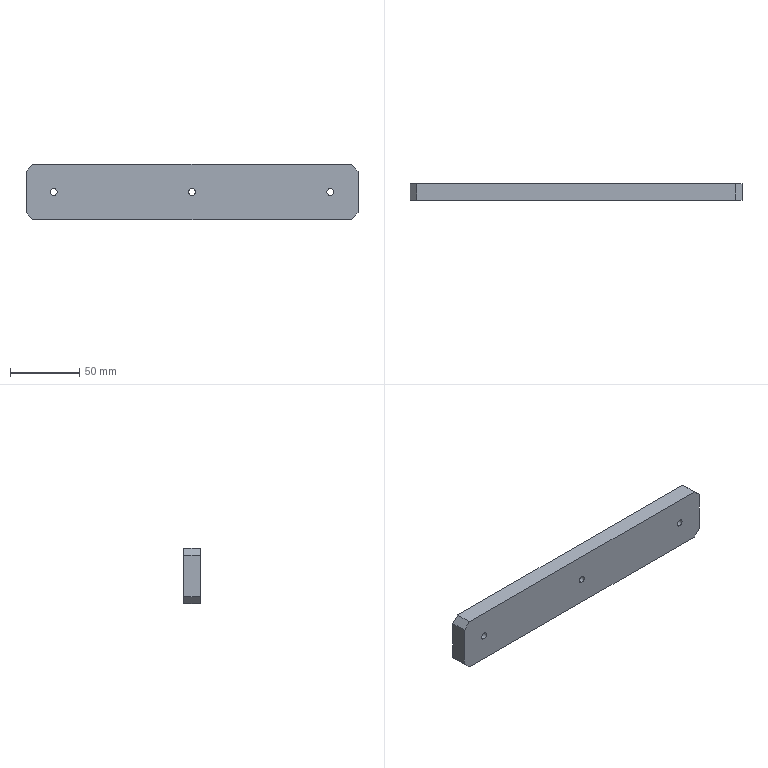Part | SolidWorks | features Chamfer 1, Extrusion 1, HoleWzd 1 | 1 solid | 16 faces | box 240 x 12 x 40 mm | volume 113893 mm3 | plane 10 | cylinder 6 | commonest cylinder face diameters 5 x6
STEP:
#1=CARTESIAN_POINT('',(-100.,-6.,-2.5));
#2=VERTEX_POINT('',#1);
#3=CARTESIAN_POINT('',(-100.,-6.,2.5));
#4=VERTEX_POINT('',#3);
#5=CARTESIAN_POINT('',(-100.,-6.,0.));
#6=DIRECTION('',(0.,1.,0.));
#7=DIRECTION('',(0.,0.,1.));
#8=AXIS2_PLACEMENT_3D('',#5,#6,#7);
#9=CIRCLE('',#8,2.5);
#10=EDGE_CURVE('',#2,#4,#9,.T.);
#11=ORIENTED_EDGE('',*,*,#10,.F.);
#12=CARTESIAN_POINT('',(-100.,6.,-2.5));
#13=VERTEX_POINT('',#12);
#14=CARTESIAN_POINT('',(-100.,6.,-2.5));
#15=DIRECTION('',(0.,1.,0.));
#16=VECTOR('',#15,1000.);
#17=LINE('',#14,#16);
#18=EDGE_CURVE('',#2,#13,#17,.T.);
#19=ORIENTED_EDGE('',*,*,#18,.T.);
#20=CARTESIAN_POINT('',(-100.,6.,2.5));
#21=VERTEX_POINT('',#20);
#22=CARTESIAN_POINT('',(-100.,6.,0.));
#23=DIRECTION('',(0.,1.,0.));
#24=DIRECTION('',(0.,0.,1.));
#25=AXIS2_PLACEMENT_3D('',#22,#23,#24);
#26=CIRCLE('',#25,2.5);
#27=EDGE_CURVE('',#13,#21,#26,.T.);
#28=ORIENTED_EDGE('',*,*,#27,.T.);
#29=CARTESIAN_POINT('',(-100.,6.,2.5));
#30=DIRECTION('',(0.,1.,0.));
#31=VECTOR('',#30,1000.);
#32=LINE('',#29,#31);
#33=EDGE_CURVE('',#4,#21,#32,.T.);
#34=ORIENTED_EDGE('',*,*,#33,.F.);
#35=EDGE_LOOP('',(#11,#19,#28,#34));
#36=FACE_OUTER_BOUND('',#35,.T.);
#37=CARTESIAN_POINT('',(-100.,6.,0.));
#38=DIRECTION('',(0.,1.,0.));
#39=DIRECTION('',(0.,0.,1.));
#40=AXIS2_PLACEMENT_3D('',#37,#38,#39);
#41=CYLINDRICAL_SURFACE('',#40,2.5);
#42=ADVANCED_FACE('',(#36),#41,.F.);
#43=CARTESIAN_POINT('',(0.,-6.,-2.5));
#44=VERTEX_POINT('',#43);
#45=CARTESIAN_POINT('',(0.,-6.,2.5));
#46=VERTEX_POINT('',#45);
#47=CARTESIAN_POINT('',(0.,-6.,0.));
#48=DIRECTION('',(0.,1.,0.));
#49=DIRECTION('',(0.,0.,1.));
#50=AXIS2_PLACEMENT_3D('',#47,#48,#49);
#51=CIRCLE('',#50,2.5);
#52=EDGE_CURVE('',#44,#46,#51,.T.);
#53=ORIENTED_EDGE('',*,*,#52,.F.);
#54=CARTESIAN_POINT('',(0.,6.,-2.5));
#55=VERTEX_POINT('',#54);
#56=CARTESIAN_POINT('',(0.,6.,-2.5));
#57=DIRECTION('',(0.,1.,0.));
#58=VECTOR('',#57,1000.);
#59=LINE('',#56,#58);
#60=EDGE_CURVE('',#44,#55,#59,.T.);
#61=ORIENTED_EDGE('',*,*,#60,.T.);
#62=CARTESIAN_POINT('',(0.,6.,2.5));
#63=VERTEX_POINT('',#62);
#64=CARTESIAN_POINT('',(0.,6.,0.));
#65=DIRECTION('',(0.,1.,0.));
#66=DIRECTION('',(0.,0.,1.));
#67=AXIS2_PLACEMENT_3D('',#64,#65,#66);
#68=CIRCLE('',#67,2.5);
#69=EDGE_CURVE('',#55,#63,#68,.T.);
#70=ORIENTED_EDGE('',*,*,#69,.T.);
#71=CARTESIAN_POINT('',(0.,6.,2.5));
#72=DIRECTION('',(0.,1.,0.));
#73=VECTOR('',#72,1000.);
#74=LINE('',#71,#73);
#75=EDGE_CURVE('',#46,#63,#74,.T.);
#76=ORIENTED_EDGE('',*,*,#75,.F.);
#77=EDGE_LOOP('',(#53,#61,#70,#76));
#78=FACE_OUTER_BOUND('',#77,.T.);
#79=CARTESIAN_POINT('',(0.,6.,0.));
#80=DIRECTION('',(0.,1.,0.));
#81=DIRECTION('',(0.,0.,1.));
#82=AXIS2_PLACEMENT_3D('',#79,#80,#81);
#83=CYLINDRICAL_SURFACE('',#82,2.5);
#84=ADVANCED_FACE('',(#78),#83,.F.);
#85=CARTESIAN_POINT('',(100.,-6.,-2.5));
#86=VERTEX_POINT('',#85);
#87=CARTESIAN_POINT('',(100.,-6.,2.5));
#88=VERTEX_POINT('',#87);
#89=CARTESIAN_POINT('',(100.,-6.,0.));
#90=DIRECTION('',(0.,1.,0.));
#91=DIRECTION('',(0.,0.,1.));
#92=AXIS2_PLACEMENT_3D('',#89,#90,#91);
#93=CIRCLE('',#92,2.5);
#94=EDGE_CURVE('',#86,#88,#93,.T.);
#95=ORIENTED_EDGE('',*,*,#94,.F.);
#96=CARTESIAN_POINT('',(100.,6.,-2.5));
#97=VERTEX_POINT('',#96);
#98=CARTESIAN_POINT('',(100.,6.,-2.5));
#99=DIRECTION('',(0.,1.,0.));
#100=VECTOR('',#99,1000.);
#101=LINE('',#98,#100);
#102=EDGE_CURVE('',#86,#97,#101,.T.);
#103=ORIENTED_EDGE('',*,*,#102,.T.);
#104=CARTESIAN_POINT('',(100.,6.,2.5));
#105=VERTEX_POINT('',#104);
#106=CARTESIAN_POINT('',(100.,6.,0.));
#107=DIRECTION('',(0.,1.,0.));
#108=DIRECTION('',(0.,0.,1.));
#109=AXIS2_PLACEMENT_3D('',#106,#107,#108);
#110=CIRCLE('',#109,2.5);
#111=EDGE_CURVE('',#97,#105,#110,.T.);
#112=ORIENTED_EDGE('',*,*,#111,.T.);
#113=CARTESIAN_POINT('',(100.,6.,2.5));
#114=DIRECTION('',(0.,1.,0.));
#115=VECTOR('',#114,1000.);
#116=LINE('',#113,#115);
#117=EDGE_CURVE('',#88,#105,#116,.T.);
#118=ORIENTED_EDGE('',*,*,#117,.F.);
#119=EDGE_LOOP('',(#95,#103,#112,#118));
#120=FACE_OUTER_BOUND('',#119,.T.);
#121=CARTESIAN_POINT('',(100.,6.,0.));
#122=DIRECTION('',(0.,1.,0.));
#123=DIRECTION('',(0.,0.,1.));
#124=AXIS2_PLACEMENT_3D('',#121,#122,#123);
#125=CYLINDRICAL_SURFACE('',#124,2.5);
#126=ADVANCED_FACE('',(#120),#125,.F.);
#127=CARTESIAN_POINT('',(-120.,-6.,-15.));
#128=VERTEX_POINT('',#127);
#129=CARTESIAN_POINT('',(-120.,-6.,15.));
#130=VERTEX_POINT('',#129);
#131=CARTESIAN_POINT('',(-120.,-6.,-20.));
#132=DIRECTION('',(0.,0.,1.));
#133=VECTOR('',#132,1000.);
#134=LINE('',#131,#133);
#135=EDGE_CURVE('',#128,#130,#134,.T.);
#136=ORIENTED_EDGE('',*,*,#135,.T.);
#137=CARTESIAN_POINT('',(-120.,6.,15.));
#138=VERTEX_POINT('',#137);
#139=CARTESIAN_POINT('',(-120.,6.,15.));
#140=DIRECTION('',(0.,1.,0.));
#141=VECTOR('',#140,1000.);
#142=LINE('',#139,#141);
#143=EDGE_CURVE('',#130,#138,#142,.T.);
#144=ORIENTED_EDGE('',*,*,#143,.T.);
#145=CARTESIAN_POINT('',(-120.,6.,-15.));
#146=VERTEX_POINT('',#145);
#147=CARTESIAN_POINT('',(-120.,6.,-20.));
#148=DIRECTION('',(0.,0.,1.));
#149=VECTOR('',#148,1000.);
#150=LINE('',#147,#149);
#151=EDGE_CURVE('',#146,#138,#150,.T.);
#152=ORIENTED_EDGE('',*,*,#151,.F.);
#153=CARTESIAN_POINT('',(-120.,6.,-15.));
#154=DIRECTION('',(0.,-1.,0.));
#155=VECTOR('',#154,1000.);
#156=LINE('',#153,#155);
#157=EDGE_CURVE('',#146,#128,#156,.T.);
#158=ORIENTED_EDGE('',*,*,#157,.T.);
#159=EDGE_LOOP('',(#136,#144,#152,#158));
#160=FACE_OUTER_BOUND('',#159,.T.);
#161=CARTESIAN_POINT('',(-120.,6.,-20.));
#162=DIRECTION('',(1.,0.,0.));
#163=DIRECTION('',(0.,0.,-1.));
#164=AXIS2_PLACEMENT_3D('',#161,#162,#163);
#165=PLANE('',#164);
#166=ADVANCED_FACE('',(#160),#165,.F.);
#167=CARTESIAN_POINT('',(-115.,-6.,20.));
#168=VERTEX_POINT('',#167);
#169=CARTESIAN_POINT('',(115.,-6.,20.));
#170=VERTEX_POINT('',#169);
#171=CARTESIAN_POINT('',(-120.,-6.,20.));
#172=DIRECTION('',(1.,0.,0.));
#173=VECTOR('',#172,1000.);
#174=LINE('',#171,#173);
#175=EDGE_CURVE('',#168,#170,#174,.T.);
#176=ORIENTED_EDGE('',*,*,#175,.T.);
#177=CARTESIAN_POINT('',(115.,6.,20.));
#178=VERTEX_POINT('',#177);
#179=CARTESIAN_POINT('',(115.,6.,20.));
#180=DIRECTION('',(0.,1.,0.));
#181=VECTOR('',#180,1000.);
#182=LINE('',#179,#181);
#183=EDGE_CURVE('',#170,#178,#182,.T.);
#184=ORIENTED_EDGE('',*,*,#183,.T.);
#185=CARTESIAN_POINT('',(-115.,6.,20.));
#186=VERTEX_POINT('',#185);
#187=CARTESIAN_POINT('',(-120.,6.,20.));
#188=DIRECTION('',(1.,0.,0.));
#189=VECTOR('',#188,1000.);
#190=LINE('',#187,#189);
#191=EDGE_CURVE('',#186,#178,#190,.T.);
#192=ORIENTED_EDGE('',*,*,#191,.F.);
#193=CARTESIAN_POINT('',(-115.,6.,20.));
#194=DIRECTION('',(0.,-1.,0.));
#195=VECTOR('',#194,1000.);
#196=LINE('',#193,#195);
#197=EDGE_CURVE('',#186,#168,#196,.T.);
#198=ORIENTED_EDGE('',*,*,#197,.T.);
#199=EDGE_LOOP('',(#176,#184,#192,#198));
#200=FACE_OUTER_BOUND('',#199,.T.);
#201=CARTESIAN_POINT('',(-120.,6.,20.));
#202=DIRECTION('',(0.,0.,-1.));
#203=DIRECTION('',(-1.,0.,0.));
#204=AXIS2_PLACEMENT_3D('',#201,#202,#203);
#205=PLANE('',#204);
#206=ADVANCED_FACE('',(#200),#205,.F.);
#207=CARTESIAN_POINT('',(120.,6.,15.));
#208=VERTEX_POINT('',#207);
#209=CARTESIAN_POINT('',(120.,6.,-15.));
#210=VERTEX_POINT('',#209);
#211=CARTESIAN_POINT('',(120.,6.,-20.));
#212=DIRECTION('',(0.,0.,-1.));
#213=VECTOR('',#212,1000.);
#214=LINE('',#211,#213);
#215=EDGE_CURVE('',#208,#210,#214,.T.);
#216=ORIENTED_EDGE('',*,*,#215,.F.);
#217=CARTESIAN_POINT('',(120.,-6.,15.));
#218=VERTEX_POINT('',#217);
#219=CARTESIAN_POINT('',(120.,6.,15.));
#220=DIRECTION('',(0.,-1.,0.));
#221=VECTOR('',#220,1000.);
#222=LINE('',#219,#221);
#223=EDGE_CURVE('',#208,#218,#222,.T.);
#224=ORIENTED_EDGE('',*,*,#223,.T.);
#225=CARTESIAN_POINT('',(120.,-6.,-15.));
#226=VERTEX_POINT('',#225);
#227=CARTESIAN_POINT('',(120.,-6.,-20.));
#228=DIRECTION('',(0.,0.,-1.));
#229=VECTOR('',#228,1000.);
#230=LINE('',#227,#229);
#231=EDGE_CURVE('',#218,#226,#230,.T.);
#232=ORIENTED_EDGE('',*,*,#231,.T.);
#233=CARTESIAN_POINT('',(120.,6.,-15.));
#234=DIRECTION('',(0.,1.,0.));
#235=VECTOR('',#234,1000.);
#236=LINE('',#233,#235);
#237=EDGE_CURVE('',#226,#210,#236,.T.);
#238=ORIENTED_EDGE('',*,*,#237,.T.);
#239=EDGE_LOOP('',(#216,#224,#232,#238));
#240=FACE_OUTER_BOUND('',#239,.T.);
#241=CARTESIAN_POINT('',(120.,6.,-20.));
#242=DIRECTION('',(-1.,0.,0.));
#243=DIRECTION('',(0.,0.,1.));
#244=AXIS2_PLACEMENT_3D('',#241,#242,#243);
#245=PLANE('',#244);
#246=ADVANCED_FACE('',(#240),#245,.F.);
#247=CARTESIAN_POINT('',(115.,-6.,-20.));
#248=VERTEX_POINT('',#247);
#249=CARTESIAN_POINT('',(-115.,-6.,-20.));
#250=VERTEX_POINT('',#249);
#251=CARTESIAN_POINT('',(-120.,-6.,-20.));
#252=DIRECTION('',(-1.,0.,0.));
#253=VECTOR('',#252,1000.);
#254=LINE('',#251,#253);
#255=EDGE_CURVE('',#248,#250,#254,.T.);
#256=ORIENTED_EDGE('',*,*,#255,.T.);
#257=CARTESIAN_POINT('',(-115.,6.,-20.));
#258=VERTEX_POINT('',#257);
#259=CARTESIAN_POINT('',(-115.,6.,-20.));
#260=DIRECTION('',(0.,1.,0.));
#261=VECTOR('',#260,1000.);
#262=LINE('',#259,#261);
#263=EDGE_CURVE('',#250,#258,#262,.T.);
#264=ORIENTED_EDGE('',*,*,#263,.T.);
#265=CARTESIAN_POINT('',(115.,6.,-20.));
#266=VERTEX_POINT('',#265);
#267=CARTESIAN_POINT('',(-120.,6.,-20.));
#268=DIRECTION('',(-1.,0.,0.));
#269=VECTOR('',#268,1000.);
#270=LINE('',#267,#269);
#271=EDGE_CURVE('',#266,#258,#270,.T.);
#272=ORIENTED_EDGE('',*,*,#271,.F.);
#273=CARTESIAN_POINT('',(115.,6.,-20.));
#274=DIRECTION('',(0.,-1.,0.));
#275=VECTOR('',#274,1000.);
#276=LINE('',#273,#275);
#277=EDGE_CURVE('',#266,#248,#276,.T.);
#278=ORIENTED_EDGE('',*,*,#277,.T.);
#279=EDGE_LOOP('',(#256,#264,#272,#278));
#280=FACE_OUTER_BOUND('',#279,.T.);
#281=CARTESIAN_POINT('',(-120.,6.,-20.));
#282=DIRECTION('',(0.,0.,1.));
#283=DIRECTION('',(1.,0.,0.));
#284=AXIS2_PLACEMENT_3D('',#281,#282,#283);
#285=PLANE('',#284);
#286=ADVANCED_FACE('',(#280),#285,.F.);
#287=CARTESIAN_POINT('',(-100.,6.,0.));
#288=DIRECTION('',(0.,1.,0.));
#289=DIRECTION('',(0.,0.,1.));
#290=AXIS2_PLACEMENT_3D('',#287,#288,#289);
#291=CIRCLE('',#290,2.5);
#292=EDGE_CURVE('',#21,#13,#291,.T.);
#293=ORIENTED_EDGE('',*,*,#292,.F.);
#294=ORIENTED_EDGE('',*,*,#27,.F.);
#295=EDGE_LOOP('',(#293,#294));
#296=FACE_BOUND('',#295,.T.);
#297=CARTESIAN_POINT('',(0.,6.,0.));
#298=DIRECTION('',(0.,1.,0.));
#299=DIRECTION('',(0.,0.,1.));
#300=AXIS2_PLACEMENT_3D('',#297,#298,#299);
#301=CIRCLE('',#300,2.5);
#302=EDGE_CURVE('',#63,#55,#301,.T.);
#303=ORIENTED_EDGE('',*,*,#302,.F.);
#304=ORIENTED_EDGE('',*,*,#69,.F.);
#305=EDGE_LOOP('',(#303,#304));
#306=FACE_BOUND('',#305,.T.);
#307=CARTESIAN_POINT('',(100.,6.,0.));
#308=DIRECTION('',(0.,1.,0.));
#309=DIRECTION('',(0.,0.,1.));
#310=AXIS2_PLACEMENT_3D('',#307,#308,#309);
#311=CIRCLE('',#310,2.5);
#312=EDGE_CURVE('',#105,#97,#311,.T.);
#313=ORIENTED_EDGE('',*,*,#312,.F.);
#314=ORIENTED_EDGE('',*,*,#111,.F.);
#315=EDGE_LOOP('',(#313,#314));
#316=FACE_BOUND('',#315,.T.);
#317=ORIENTED_EDGE('',*,*,#191,.T.);
#318=CARTESIAN_POINT('',(-2.5,6.,137.5));
#319=DIRECTION('',(0.7071,0.,-0.7071));
#320=VECTOR('',#319,1000.);
#321=LINE('',#318,#320);
#322=EDGE_CURVE('',#178,#208,#321,.T.);
#323=ORIENTED_EDGE('',*,*,#322,.T.);
#324=ORIENTED_EDGE('',*,*,#215,.T.);
#325=CARTESIAN_POINT('',(17.5,6.,-117.5));
#326=DIRECTION('',(-0.7071,0.,-0.7071));
#327=VECTOR('',#326,1000.);
#328=LINE('',#325,#327);
#329=EDGE_CURVE('',#210,#266,#328,.T.);
#330=ORIENTED_EDGE('',*,*,#329,.T.);
#331=ORIENTED_EDGE('',*,*,#271,.T.);
#332=CARTESIAN_POINT('',(-137.5,6.,2.5));
#333=DIRECTION('',(-0.7071,0.,0.7071));
#334=VECTOR('',#333,1000.);
#335=LINE('',#332,#334);
#336=EDGE_CURVE('',#258,#146,#335,.T.);
#337=ORIENTED_EDGE('',*,*,#336,.T.);
#338=ORIENTED_EDGE('',*,*,#151,.T.);
#339=CARTESIAN_POINT('',(-117.5,6.,17.5));
#340=DIRECTION('',(0.7071,0.,0.7071));
#341=VECTOR('',#340,1000.);
#342=LINE('',#339,#341);
#343=EDGE_CURVE('',#138,#186,#342,.T.);
#344=ORIENTED_EDGE('',*,*,#343,.T.);
#345=EDGE_LOOP('',(#317,#323,#324,#330,#331,#337,#338,#344));
#346=FACE_OUTER_BOUND('',#345,.T.);
#347=CARTESIAN_POINT('',(-120.,6.,20.));
#348=DIRECTION('',(0.,1.,0.));
#349=DIRECTION('',(0.,0.,1.));
#350=AXIS2_PLACEMENT_3D('',#347,#348,#349);
#351=PLANE('',#350);
#352=ADVANCED_FACE('',(#296,#306,#316,#346),#351,.T.);
#353=CARTESIAN_POINT('',(-100.,-6.,0.));
#354=DIRECTION('',(0.,1.,0.));
#355=DIRECTION('',(0.,0.,1.));
#356=AXIS2_PLACEMENT_3D('',#353,#354,#355);
#357=CIRCLE('',#356,2.5);
#358=EDGE_CURVE('',#4,#2,#357,.T.);
#359=ORIENTED_EDGE('',*,*,#358,.T.);
#360=ORIENTED_EDGE('',*,*,#10,.T.);
#361=EDGE_LOOP('',(#359,#360));
#362=FACE_BOUND('',#361,.T.);
#363=CARTESIAN_POINT('',(0.,-6.,0.));
#364=DIRECTION('',(0.,1.,0.));
#365=DIRECTION('',(0.,0.,1.));
#366=AXIS2_PLACEMENT_3D('',#363,#364,#365);
#367=CIRCLE('',#366,2.5);
#368=EDGE_CURVE('',#46,#44,#367,.T.);
#369=ORIENTED_EDGE('',*,*,#368,.T.);
#370=ORIENTED_EDGE('',*,*,#52,.T.);
#371=EDGE_LOOP('',(#369,#370));
#372=FACE_BOUND('',#371,.T.);
#373=CARTESIAN_POINT('',(100.,-6.,0.));
#374=DIRECTION('',(0.,1.,0.));
#375=DIRECTION('',(0.,0.,1.));
#376=AXIS2_PLACEMENT_3D('',#373,#374,#375);
#377=CIRCLE('',#376,2.5);
#378=EDGE_CURVE('',#88,#86,#377,.T.);
#379=ORIENTED_EDGE('',*,*,#378,.T.);
#380=ORIENTED_EDGE('',*,*,#94,.T.);
#381=EDGE_LOOP('',(#379,#380));
#382=FACE_BOUND('',#381,.T.);
#383=ORIENTED_EDGE('',*,*,#231,.F.);
#384=CARTESIAN_POINT('',(120.,-6.,15.));
#385=DIRECTION('',(-0.7071,0.,0.7071));
#386=VECTOR('',#385,1000.);
#387=LINE('',#384,#386);
#388=EDGE_CURVE('',#218,#170,#387,.T.);
#389=ORIENTED_EDGE('',*,*,#388,.T.);
#390=ORIENTED_EDGE('',*,*,#175,.F.);
#391=CARTESIAN_POINT('',(-115.,-6.,20.));
#392=DIRECTION('',(-0.7071,0.,-0.7071));
#393=VECTOR('',#392,1000.);
#394=LINE('',#391,#393);
#395=EDGE_CURVE('',#168,#130,#394,.T.);
#396=ORIENTED_EDGE('',*,*,#395,.T.);
#397=ORIENTED_EDGE('',*,*,#135,.F.);
#398=CARTESIAN_POINT('',(-120.,-6.,-15.));
#399=DIRECTION('',(0.7071,0.,-0.7071));
#400=VECTOR('',#399,1000.);
#401=LINE('',#398,#400);
#402=EDGE_CURVE('',#128,#250,#401,.T.);
#403=ORIENTED_EDGE('',*,*,#402,.T.);
#404=ORIENTED_EDGE('',*,*,#255,.F.);
#405=CARTESIAN_POINT('',(115.,-6.,-20.));
#406=DIRECTION('',(0.7071,0.,0.7071));
#407=VECTOR('',#406,1000.);
#408=LINE('',#405,#407);
#409=EDGE_CURVE('',#248,#226,#408,.T.);
#410=ORIENTED_EDGE('',*,*,#409,.T.);
#411=EDGE_LOOP('',(#383,#389,#390,#396,#397,#403,#404,#410));
#412=FACE_OUTER_BOUND('',#411,.T.);
#413=CARTESIAN_POINT('',(-120.,-6.,20.));
#414=DIRECTION('',(0.,1.,0.));
#415=DIRECTION('',(0.,0.,1.));
#416=AXIS2_PLACEMENT_3D('',#413,#414,#415);
#417=PLANE('',#416);
#418=ADVANCED_FACE('',(#362,#372,#382,#412),#417,.F.);
#419=ORIENTED_EDGE('',*,*,#102,.F.);
#420=ORIENTED_EDGE('',*,*,#378,.F.);
#421=ORIENTED_EDGE('',*,*,#117,.T.);
#422=ORIENTED_EDGE('',*,*,#312,.T.);
#423=EDGE_LOOP('',(#419,#420,#421,#422));
#424=FACE_OUTER_BOUND('',#423,.T.);
#425=CARTESIAN_POINT('',(100.,6.,0.));
#426=DIRECTION('',(0.,1.,0.));
#427=DIRECTION('',(0.,0.,1.));
#428=AXIS2_PLACEMENT_3D('',#425,#426,#427);
#429=CYLINDRICAL_SURFACE('',#428,2.5);
#430=ADVANCED_FACE('',(#424),#429,.F.);
#431=ORIENTED_EDGE('',*,*,#60,.F.);
#432=ORIENTED_EDGE('',*,*,#368,.F.);
#433=ORIENTED_EDGE('',*,*,#75,.T.);
#434=ORIENTED_EDGE('',*,*,#302,.T.);
#435=EDGE_LOOP('',(#431,#432,#433,#434));
#436=FACE_OUTER_BOUND('',#435,.T.);
#437=CARTESIAN_POINT('',(0.,6.,0.));
#438=DIRECTION('',(0.,1.,0.));
#439=DIRECTION('',(0.,0.,1.));
#440=AXIS2_PLACEMENT_3D('',#437,#438,#439);
#441=CYLINDRICAL_SURFACE('',#440,2.5);
#442=ADVANCED_FACE('',(#436),#441,.F.);
#443=ORIENTED_EDGE('',*,*,#18,.F.);
#444=ORIENTED_EDGE('',*,*,#358,.F.);
#445=ORIENTED_EDGE('',*,*,#33,.T.);
#446=ORIENTED_EDGE('',*,*,#292,.T.);
#447=EDGE_LOOP('',(#443,#444,#445,#446));
#448=FACE_OUTER_BOUND('',#447,.T.);
#449=CARTESIAN_POINT('',(-100.,6.,0.));
#450=DIRECTION('',(0.,1.,0.));
#451=DIRECTION('',(0.,0.,1.));
#452=AXIS2_PLACEMENT_3D('',#449,#450,#451);
#453=CYLINDRICAL_SURFACE('',#452,2.5);
#454=ADVANCED_FACE('',(#448),#453,.F.);
#455=ORIENTED_EDGE('',*,*,#322,.F.);
#456=ORIENTED_EDGE('',*,*,#183,.F.);
#457=ORIENTED_EDGE('',*,*,#388,.F.);
#458=ORIENTED_EDGE('',*,*,#223,.F.);
#459=EDGE_LOOP('',(#455,#456,#457,#458));
#460=FACE_OUTER_BOUND('',#459,.T.);
#461=CARTESIAN_POINT('',(120.,6.,15.));
#462=DIRECTION('',(-0.7071,0.,-0.7071));
#463=DIRECTION('',(-0.7071,0.,0.7071));
#464=AXIS2_PLACEMENT_3D('',#461,#462,#463);
#465=PLANE('',#464);
#466=ADVANCED_FACE('',(#460),#465,.F.);
#467=ORIENTED_EDGE('',*,*,#343,.F.);
#468=ORIENTED_EDGE('',*,*,#143,.F.);
#469=ORIENTED_EDGE('',*,*,#395,.F.);
#470=ORIENTED_EDGE('',*,*,#197,.F.);
#471=EDGE_LOOP('',(#467,#468,#469,#470));
#472=FACE_OUTER_BOUND('',#471,.T.);
#473=CARTESIAN_POINT('',(-115.,6.,20.));
#474=DIRECTION('',(0.7071,0.,-0.7071));
#475=DIRECTION('',(-0.7071,0.,-0.7071));
#476=AXIS2_PLACEMENT_3D('',#473,#474,#475);
#477=PLANE('',#476);
#478=ADVANCED_FACE('',(#472),#477,.F.);
#479=ORIENTED_EDGE('',*,*,#336,.F.);
#480=ORIENTED_EDGE('',*,*,#263,.F.);
#481=ORIENTED_EDGE('',*,*,#402,.F.);
#482=ORIENTED_EDGE('',*,*,#157,.F.);
#483=EDGE_LOOP('',(#479,#480,#481,#482));
#484=FACE_OUTER_BOUND('',#483,.T.);
#485=CARTESIAN_POINT('',(-120.,6.,-15.));
#486=DIRECTION('',(0.7071,0.,0.7071));
#487=DIRECTION('',(0.7071,0.,-0.7071));
#488=AXIS2_PLACEMENT_3D('',#485,#486,#487);
#489=PLANE('',#488);
#490=ADVANCED_FACE('',(#484),#489,.F.);
#491=ORIENTED_EDGE('',*,*,#329,.F.);
#492=ORIENTED_EDGE('',*,*,#237,.F.);
#493=ORIENTED_EDGE('',*,*,#409,.F.);
#494=ORIENTED_EDGE('',*,*,#277,.F.);
#495=EDGE_LOOP('',(#491,#492,#493,#494));
#496=FACE_OUTER_BOUND('',#495,.T.);
#497=CARTESIAN_POINT('',(115.,6.,-20.));
#498=DIRECTION('',(-0.7071,0.,0.7071));
#499=DIRECTION('',(0.7071,0.,0.7071));
#500=AXIS2_PLACEMENT_3D('',#497,#498,#499);
#501=PLANE('',#500);
#502=ADVANCED_FACE('',(#496),#501,.F.);
#503=CLOSED_SHELL('',(#42,#84,#126,#166,#206,#246,#286,#352,#418,#430,#442,#454,#466,#478,#490,#502));
#504=MANIFOLD_SOLID_BREP('',#503);
#505=CARTESIAN_POINT('',(0.,0.,0.));
#506=DIRECTION('',(0.,0.,1.));
#507=DIRECTION('',(1.,0.,0.));
#508=AXIS2_PLACEMENT_3D('',#505,#506,#507);
#509=(LENGTH_UNIT()NAMED_UNIT(*)SI_UNIT(.MILLI.,.METRE.));
#510=UNCERTAINTY_MEASURE_WITH_UNIT(LENGTH_MEASURE(0.00001),#509,'','');
#511=(NAMED_UNIT(*)PLANE_ANGLE_UNIT()SI_UNIT($,.RADIAN.));
#512=(NAMED_UNIT(*)SI_UNIT($,.STERADIAN.)SOLID_ANGLE_UNIT());
#513=(GEOMETRIC_REPRESENTATION_CONTEXT(3)GLOBAL_UNCERTAINTY_ASSIGNED_CONTEXT((#510))GLOBAL_UNIT_ASSIGNED_CONTEXT((#509,#511,#512))REPRESENTATION_CONTEXT('',''));
#514=ADVANCED_BREP_SHAPE_REPRESENTATION('',(#504,#508),#513);